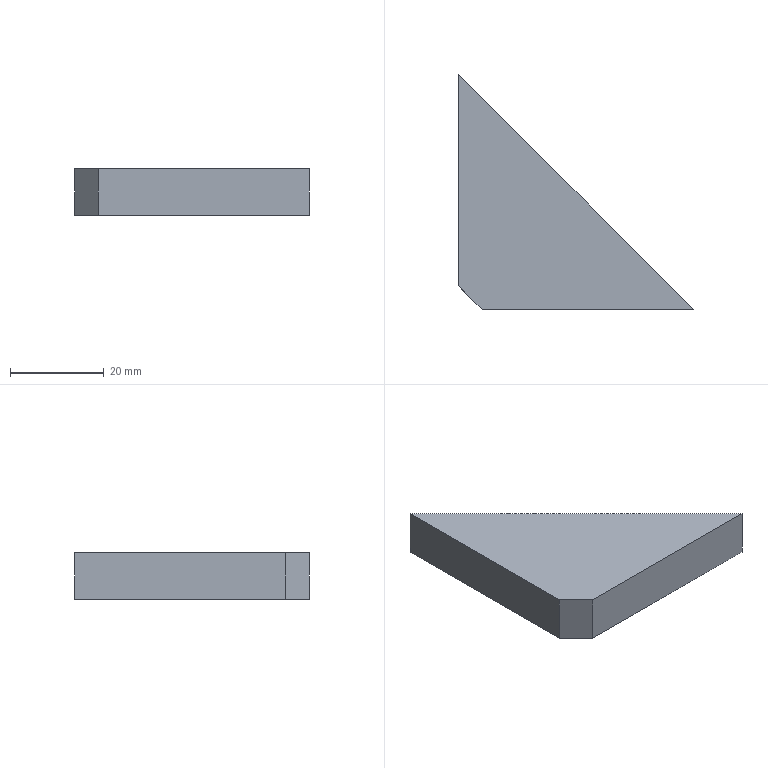Part | SolidWorks | features Chamfer 1, Extrusion 1 | 1 solid | 6 faces | box 50 x 50 x 10 mm | volume 12375 mm3 | plane 6
STEP:
#1=CARTESIAN_POINT('',(5.,0.,5.));
#2=VERTEX_POINT('',#1);
#3=CARTESIAN_POINT('',(50.,0.,5.));
#4=VERTEX_POINT('',#3);
#5=CARTESIAN_POINT('',(50.,0.,5.));
#6=DIRECTION('',(1.,0.,0.));
#7=VECTOR('',#6,1000.);
#8=LINE('',#5,#7);
#9=EDGE_CURVE('',#2,#4,#8,.T.);
#10=ORIENTED_EDGE('',*,*,#9,.F.);
#11=CARTESIAN_POINT('',(5.,0.,-5.));
#12=VERTEX_POINT('',#11);
#13=CARTESIAN_POINT('',(5.,0.,5.));
#14=DIRECTION('',(0.,0.,-1.));
#15=VECTOR('',#14,1000.);
#16=LINE('',#13,#15);
#17=EDGE_CURVE('',#2,#12,#16,.T.);
#18=ORIENTED_EDGE('',*,*,#17,.T.);
#19=CARTESIAN_POINT('',(50.,0.,-5.));
#20=VERTEX_POINT('',#19);
#21=CARTESIAN_POINT('',(50.,0.,-5.));
#22=DIRECTION('',(1.,0.,0.));
#23=VECTOR('',#22,1000.);
#24=LINE('',#21,#23);
#25=EDGE_CURVE('',#12,#20,#24,.T.);
#26=ORIENTED_EDGE('',*,*,#25,.T.);
#27=CARTESIAN_POINT('',(50.,0.,5.));
#28=DIRECTION('',(0.,0.,-1.));
#29=VECTOR('',#28,1000.);
#30=LINE('',#27,#29);
#31=EDGE_CURVE('',#4,#20,#30,.T.);
#32=ORIENTED_EDGE('',*,*,#31,.F.);
#33=EDGE_LOOP('',(#10,#18,#26,#32));
#34=FACE_OUTER_BOUND('',#33,.T.);
#35=CARTESIAN_POINT('',(50.,0.,5.));
#36=DIRECTION('',(0.,1.,0.));
#37=DIRECTION('',(0.,0.,1.));
#38=AXIS2_PLACEMENT_3D('',#35,#36,#37);
#39=PLANE('',#38);
#40=ADVANCED_FACE('',(#34),#39,.F.);
#41=CARTESIAN_POINT('',(0.,50.,-5.));
#42=VERTEX_POINT('',#41);
#43=CARTESIAN_POINT('',(0.,50.,-5.));
#44=DIRECTION('',(-0.7071,0.7071,0.));
#45=VECTOR('',#44,1000.);
#46=LINE('',#43,#45);
#47=EDGE_CURVE('',#20,#42,#46,.T.);
#48=ORIENTED_EDGE('',*,*,#47,.T.);
#49=CARTESIAN_POINT('',(0.,50.,5.));
#50=VERTEX_POINT('',#49);
#51=CARTESIAN_POINT('',(0.,50.,5.));
#52=DIRECTION('',(0.,0.,-1.));
#53=VECTOR('',#52,1000.);
#54=LINE('',#51,#53);
#55=EDGE_CURVE('',#50,#42,#54,.T.);
#56=ORIENTED_EDGE('',*,*,#55,.F.);
#57=CARTESIAN_POINT('',(0.,50.,5.));
#58=DIRECTION('',(-0.7071,0.7071,0.));
#59=VECTOR('',#58,1000.);
#60=LINE('',#57,#59);
#61=EDGE_CURVE('',#4,#50,#60,.T.);
#62=ORIENTED_EDGE('',*,*,#61,.F.);
#63=ORIENTED_EDGE('',*,*,#31,.T.);
#64=EDGE_LOOP('',(#48,#56,#62,#63));
#65=FACE_OUTER_BOUND('',#64,.T.);
#66=CARTESIAN_POINT('',(0.,50.,5.));
#67=DIRECTION('',(-0.7071,-0.7071,0.));
#68=DIRECTION('',(0.7071,-0.7071,0.));
#69=AXIS2_PLACEMENT_3D('',#66,#67,#68);
#70=PLANE('',#69);
#71=ADVANCED_FACE('',(#65),#70,.F.);
#72=CARTESIAN_POINT('',(0.,5.,-5.));
#73=VERTEX_POINT('',#72);
#74=CARTESIAN_POINT('',(0.,0.,-5.));
#75=DIRECTION('',(0.,-1.,0.));
#76=VECTOR('',#75,1000.);
#77=LINE('',#74,#76);
#78=EDGE_CURVE('',#42,#73,#77,.T.);
#79=ORIENTED_EDGE('',*,*,#78,.T.);
#80=CARTESIAN_POINT('',(0.,5.,5.));
#81=VERTEX_POINT('',#80);
#82=CARTESIAN_POINT('',(0.,5.,5.));
#83=DIRECTION('',(0.,0.,1.));
#84=VECTOR('',#83,1000.);
#85=LINE('',#82,#84);
#86=EDGE_CURVE('',#73,#81,#85,.T.);
#87=ORIENTED_EDGE('',*,*,#86,.T.);
#88=CARTESIAN_POINT('',(0.,0.,5.));
#89=DIRECTION('',(0.,-1.,0.));
#90=VECTOR('',#89,1000.);
#91=LINE('',#88,#90);
#92=EDGE_CURVE('',#50,#81,#91,.T.);
#93=ORIENTED_EDGE('',*,*,#92,.F.);
#94=ORIENTED_EDGE('',*,*,#55,.T.);
#95=EDGE_LOOP('',(#79,#87,#93,#94));
#96=FACE_OUTER_BOUND('',#95,.T.);
#97=CARTESIAN_POINT('',(0.,0.,5.));
#98=DIRECTION('',(1.,0.,0.));
#99=DIRECTION('',(0.,0.,-1.));
#100=AXIS2_PLACEMENT_3D('',#97,#98,#99);
#101=PLANE('',#100);
#102=ADVANCED_FACE('',(#96),#101,.F.);
#103=ORIENTED_EDGE('',*,*,#92,.T.);
#104=CARTESIAN_POINT('',(5.,0.,5.));
#105=DIRECTION('',(0.7071,-0.7071,0.));
#106=VECTOR('',#105,1000.);
#107=LINE('',#104,#106);
#108=EDGE_CURVE('',#81,#2,#107,.T.);
#109=ORIENTED_EDGE('',*,*,#108,.T.);
#110=ORIENTED_EDGE('',*,*,#9,.T.);
#111=ORIENTED_EDGE('',*,*,#61,.T.);
#112=EDGE_LOOP('',(#103,#109,#110,#111));
#113=FACE_OUTER_BOUND('',#112,.T.);
#114=CARTESIAN_POINT('',(0.,0.,5.));
#115=DIRECTION('',(0.,0.,-1.));
#116=DIRECTION('',(-1.,0.,0.));
#117=AXIS2_PLACEMENT_3D('',#114,#115,#116);
#118=PLANE('',#117);
#119=ADVANCED_FACE('',(#113),#118,.F.);
#120=ORIENTED_EDGE('',*,*,#25,.F.);
#121=CARTESIAN_POINT('',(2.5,2.5,-5.));
#122=DIRECTION('',(-0.7071,0.7071,0.));
#123=VECTOR('',#122,1000.);
#124=LINE('',#121,#123);
#125=EDGE_CURVE('',#12,#73,#124,.T.);
#126=ORIENTED_EDGE('',*,*,#125,.T.);
#127=ORIENTED_EDGE('',*,*,#78,.F.);
#128=ORIENTED_EDGE('',*,*,#47,.F.);
#129=EDGE_LOOP('',(#120,#126,#127,#128));
#130=FACE_OUTER_BOUND('',#129,.T.);
#131=CARTESIAN_POINT('',(0.,0.,-5.));
#132=DIRECTION('',(0.,0.,-1.));
#133=DIRECTION('',(-1.,0.,0.));
#134=AXIS2_PLACEMENT_3D('',#131,#132,#133);
#135=PLANE('',#134);
#136=ADVANCED_FACE('',(#130),#135,.T.);
#137=ORIENTED_EDGE('',*,*,#108,.F.);
#138=ORIENTED_EDGE('',*,*,#86,.F.);
#139=ORIENTED_EDGE('',*,*,#125,.F.);
#140=ORIENTED_EDGE('',*,*,#17,.F.);
#141=EDGE_LOOP('',(#137,#138,#139,#140));
#142=FACE_OUTER_BOUND('',#141,.T.);
#143=CARTESIAN_POINT('',(5.,0.,5.));
#144=DIRECTION('',(0.7071,0.7071,0.));
#145=DIRECTION('',(0.,0.,-1.));
#146=AXIS2_PLACEMENT_3D('',#143,#144,#145);
#147=PLANE('',#146);
#148=ADVANCED_FACE('',(#142),#147,.F.);
#149=CLOSED_SHELL('',(#40,#71,#102,#119,#136,#148));
#150=MANIFOLD_SOLID_BREP('',#149);
#151=CARTESIAN_POINT('',(0.,0.,0.));
#152=DIRECTION('',(0.,0.,1.));
#153=DIRECTION('',(1.,0.,0.));
#154=AXIS2_PLACEMENT_3D('',#151,#152,#153);
#155=(LENGTH_UNIT()NAMED_UNIT(*)SI_UNIT(.MILLI.,.METRE.));
#156=UNCERTAINTY_MEASURE_WITH_UNIT(LENGTH_MEASURE(0.00001),#155,'','');
#157=(NAMED_UNIT(*)PLANE_ANGLE_UNIT()SI_UNIT($,.RADIAN.));
#158=(NAMED_UNIT(*)SI_UNIT($,.STERADIAN.)SOLID_ANGLE_UNIT());
#159=(GEOMETRIC_REPRESENTATION_CONTEXT(3)GLOBAL_UNCERTAINTY_ASSIGNED_CONTEXT((#156))GLOBAL_UNIT_ASSIGNED_CONTEXT((#155,#157,#158))REPRESENTATION_CONTEXT('',''));
#160=ADVANCED_BREP_SHAPE_REPRESENTATION('',(#150,#154),#159);